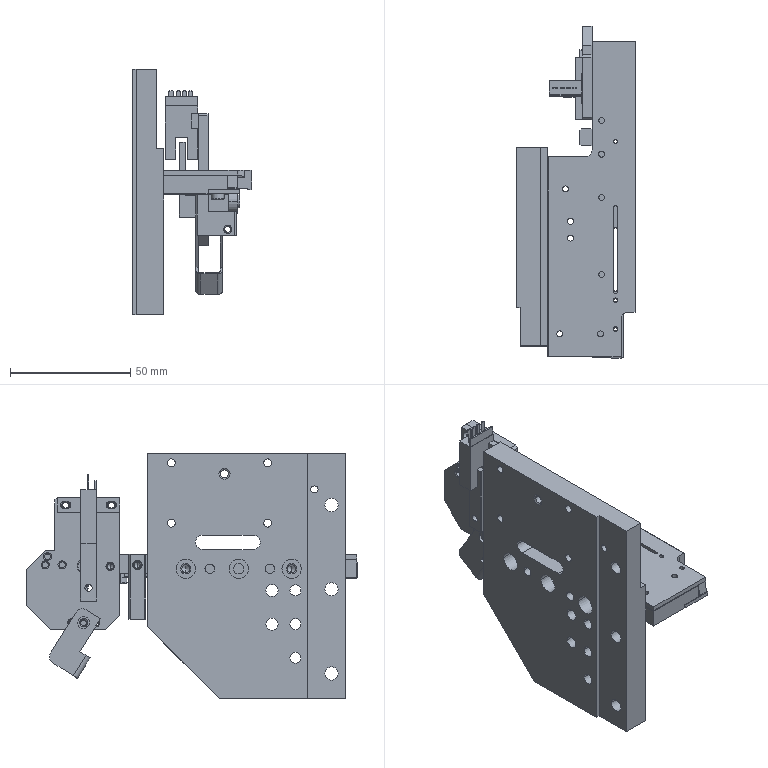Part | NX | 19 solids | 1272 faces | box 49.55 x 138 x 102 mm | volume 132627 mm3 | plane 890 | cylinder 244 | cone 130 | torus 8 | commonest cylinder face diameters 2.5 x61 3 x22 4 x18 5.5 x18 1.5 x15 3.3 x14